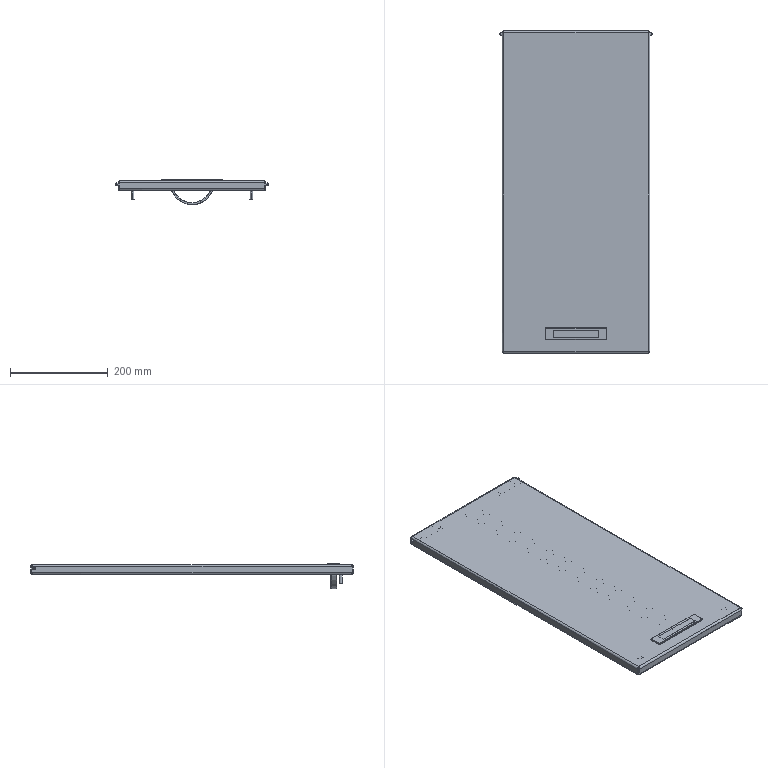Part | NX | features BREP 11 | 12 solids | 434 faces | box 312 x 659 x 52 mm | volume 594578 mm3 | plane 180 | cylinder 124 | torus 94 | cone 20 | spline 16 | commonest cylinder face diameters 6 x20 10 x16 4 x14 7 x12 8 x12 2 x8